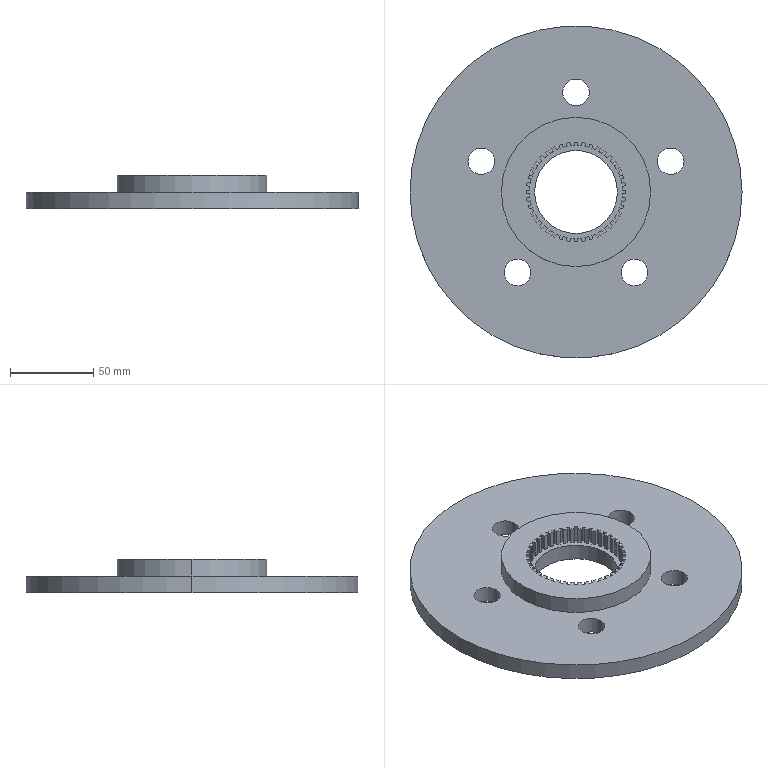Part | SolidWorks | features Extrusion 1, ICE 1 | 1 solid | 180 faces | box 200 x 200 x 20 mm | volume 321867 mm3 | plane 124 | cylinder 56 | commonest cylinder face diameters 56 x40 16 x10 50 x2 90 x2 200 x2